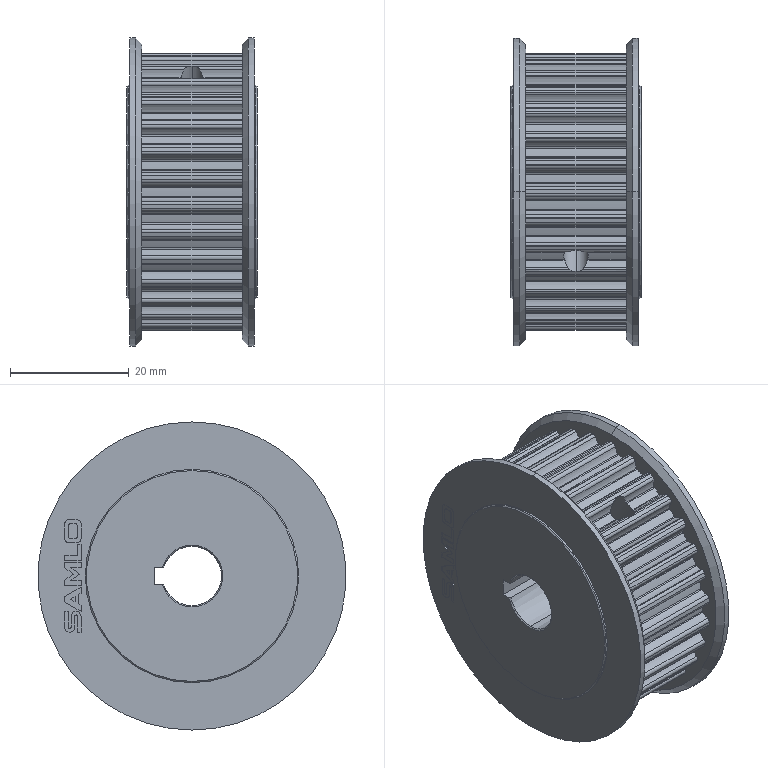Part | SolidWorks | features BaseBody 1 | 1 solid | 383 faces | box 22 x 52 x 52 mm | volume 33852 mm3 | cylinder 305 | plane 64 | cone 14 | commonest cylinder face diameters 1.1 x73 0.5 x72 6.55 x68 43.25 x32 46.79 x31 0.643 x4